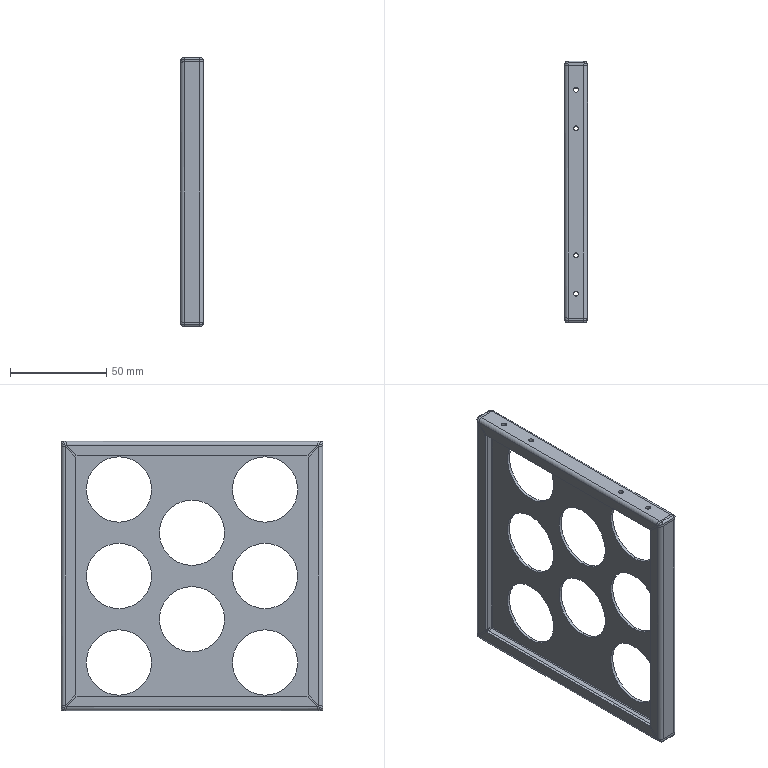Part | SolidWorks | features SMWeldBead 4, EdgeFlange 2, FlatPattern 1, HoleWzd 1, ICE 1, LPattern 1, SMBaseFlange 1, SheetMetal 1 | 1 solid | 146 faces | box 12 x 136 x 140 mm | volume 29958 mm3 | plane 54 | cylinder 52 | spline 40 | commonest cylinder face diameters 2.5 x16 34 x16 1 x8 4 x8 2 x4